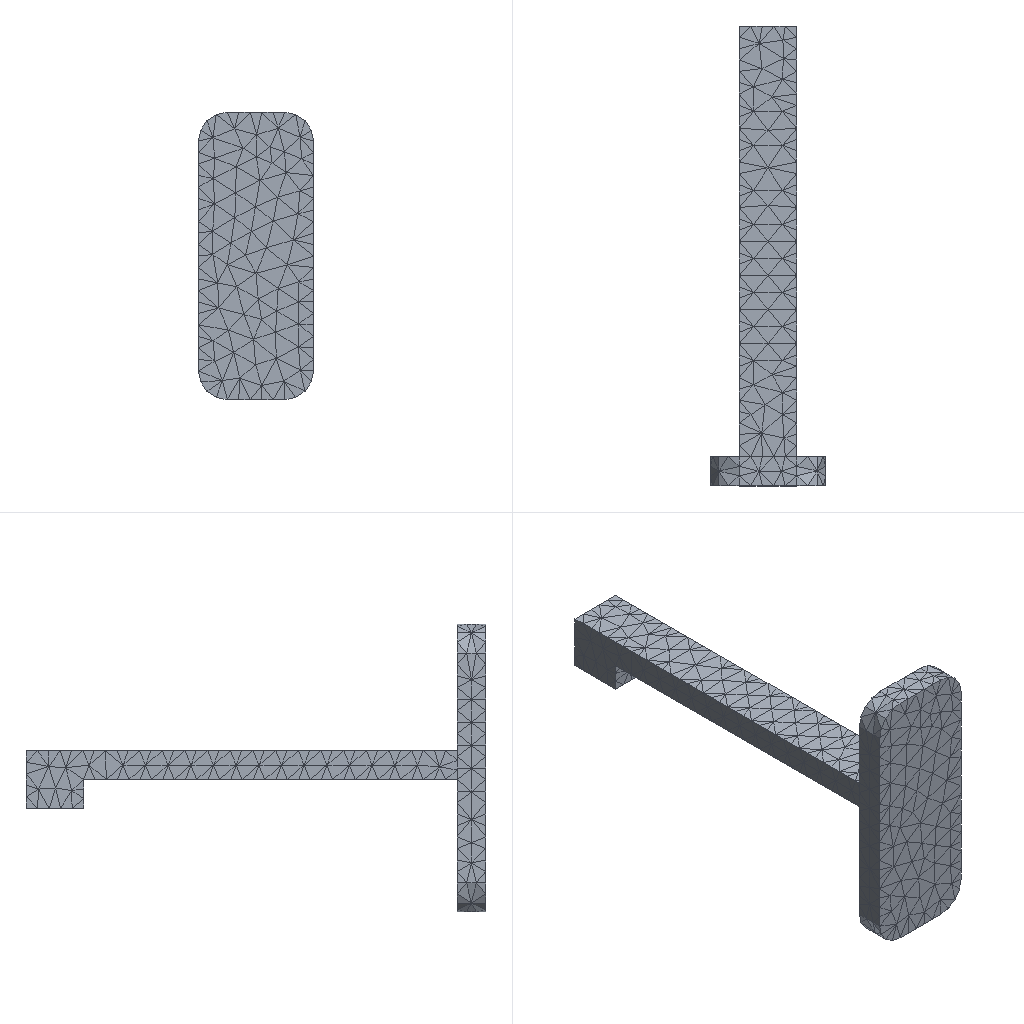Simulation study | ansys workbench
Ansys APDL input file, long lists of numbers shortened:
/batch
/config,noeldb,1     ! force off writing results to database
*get,_wallstrt,active,,time,wall
! ANSYS input file written by Workbench version 2021 R1
! File used for geometry attach:
/title,111111--____ (A5)
! ****** Begin Custom Load Command Snippet ******
/COM, ACT Extensions:
/COM,     LSDYNA, 2021.1
/COM,
! ****** End   Custom Load Command Snippet ******
*DIM,_wb_ProjectScratch_dir,string,248
_wb_ProjectScratch_dir(1) = ''
*DIM,_wb_SolverFiles_dir,string,248
_wb_SolverFiles_dir(1) = ''
*DIM,_wb_userfiles_dir,string,248
_wb_userfiles_dir(1) = ''
/com,--- Data in consistent NMM units. See Solving Units in the help system for more information.
/units,MPA
/nopr
/wb,file,start              !  signify a WB generated input file
/prep7
! Turn off shape checking because checks already performed inside WB mesher.
! See help system for more information.
SHPP,OFF,,NOWARN
/nolist
etcon,set             ! allow ANSYS to choose best KEYOP's for 180x elements, resets any applicable keyopt to MAPDL defaults
/com,*********** Nodes for the whole assembly ***********
nblock,3,,4436
(1i9,3e20.9e3)
        1     5.000000000E+00     8.000000000E+01    -3.200000000E+01
! (4032 more lines like these left out)
-1
/wb,elem,start            !  set before creation of elements
/com,*********** Elements for Body 1 "SYS-2\__" ***********
et,1,187
eblock,19,solid,,1982
(19i9)
        1        1        1        1        0        0        0        0       10        0        1      543      588      719      661     3482     3718     3487     3483
! (3963 more lines like these left out)
-1
/wb,elem,end               !  done creating elements
/com,*********** Send User Defined Coordinate System(s) ***********
csys,0
toffst,273.15,  ! Temperature offset from absolute zero
/com,*********** Set Reference Temperature ***********
tref,22.
/wb,mat,start              !  starting to send materials
/com,*********** Send Materials ***********
Temperature = 'TEMP' ! Temperature
MP,DENS,1,7.85e-09,	! tonne mm^-3
MP,ALPX,1,1.2e-05,	! C^-1
MP,C,1,434000000,	! mm^2 s^-2 C^-1
MP,KXX,1,60.5,	! tonne mm s^-3 C^-1
MP,RSVX,1,0.00017,	! ohm mm
MP,EX,1,200000,	! tonne s^-2 mm^-1
MP,NUXY,1,0.3,
MP,MURX,1,10000,
/wb,mat,end                !  done sending materials
!************************* Model Summary ********************
!SYS-2\__,	304,	matid,	1
!************************* End Model Summary ********************
! get the diagonal of the bounding box. Needed later for other things
*get,_xmin,node,,mnloc,x
*get,_ymin,node,,mnloc,y
*get,_zmin,node,,mnloc,z
*get,_xmax,node,,mxloc,x
*get,_ymax,node,,mxloc,y
*get,_zmax,node,,mxloc,z
_ASMDIAG=(_xmax-_xmin)*(_xmax-_xmin)+(_ymax-_ymin)*(_ymax-_ymin)+(_zmax-_zmin)*(_zmax-_zmin)
_ASMDIAG=SQRT(_ASMDIAG)
/wb,contact,start          !  starting to send contact
/wb,contact,end            !  done creating contacts
/golist
/wb,load,start             !  starting to send loads
/com,*********** Fixed Supports ***********
CMBLOCK,_FIXEDSU,NODE,      431
(8i10)
       265       268       269       270       271       272       275       278
! (53 more lines like these left out)
cmsel,s,_FIXEDSU
d,all,all
nsel,all
/com,*********** Define Force Using Surface Effect Elements ***********
local,12,0,0.,0.,0.,0.,0.,0.
csys,0
et,2,154
eblock,10,,,28
(15i9)
     3211        2        2        2       12        9      578      579      579      760     3650      579      761
! (27 more lines like these left out)
-1
esel,s,type,,2
keyop,2,2,1                ! Apply load in local coordinate system
keyop,2,7,1                ! Use original area so load is constant in large deformation
esel,all
/gst,on,on
fini
*get,_numnode,node,0,count
*get,_numelem,elem,0,count
*get, _MAXELEMNUM, elem, 0, NUM, MAX
*get, _MAXNODENUM, node, 0, NUM, MAX
*get, _MAXELEMTYPE, etyp, 0, NUM, MAX
*get, _MAXREALCONST, real, 0, NUM, MAX
/go
/wb,load,end               !  done creating loads
/com,--- Number of total nodes = %_numnode%
/com,--- Number of contact elements = 28
/com,--- Number of spring elements = 0
/com,--- Number of bearing elements = 0
/com,--- Number of solid elements = 1982
/com,--- Number of condensed parts = 0
/com,--- Number of total elements = %_numelem%
*get,_wallbsol,active,,time,wall
/com,****************************************************************************
/com,*************************    SOLUTION       ********************************
/com,****************************************************************************
/solu
antype,0                   ! static analysis
_thickRatio=  0     ! Ratio of thick parts in the model
eqsl,sparse,,,,,1
cntr,print,1               ! print out contact info and also make no initial contact an error
dmpoption,emat,no             ! Don't combine emat file for DANSYS
dmpoption,esav,no             ! Don't combine esav file for DANSYS
nldiag,cont,iter           ! print out contact info each equilibrium iteration
rescontrol,,none                 ! Do not keep any restart files
/com,****************************************************
/com,******************* SOLVE FOR LS 1 OF 1 ****************
esel,s,type,,2
nsle
sfe,all,1,pres,1,0.
sfe,all,2,pres,1,0.
sfe,all,3,pres,1,5.
nsel,all
esel,all
/nopr
/gopr
/nolist
nsub,1,1,1
time,1.
outres,erase
outres,all,none
outres,nsol,all,
outres,rsol,all
outres,eangl,all
outres,etmp,all
outres,veng,all
outres,strs,all,
outres,epel,all,
outres,eppl,all,
outres,cont,all,
! *********** WB SOLVE COMMAND ***********
! check interactive state
*get,ANSINTER_,active,,int
*if,ANSINTER_,ne,0,then
/eof
*endif
solve
/com *************** Write FE CONNECTORS *********
CEWRITE,file,ce,,INTE
/com,****************************************************
/com,*************** FINISHED SOLVE FOR LS 1 *************
*get,_wallasol,active,,time,wall
/nopr
*get,_numnode,node,0,count
*get,_numelem,elem,0,count
*get, _MAXELEMNUM, elem, 0, NUM, MAX
*get, _MAXNODENUM, node, 0, NUM, MAX,,,INTERNAL
*get, _MAXELEMTYPE, etyp, 0, NUM, MAX
*get, _MAXREALCONST, real, 0, NUM, MAX
/gopr
/post1
xmlo,ENCODING,ISO-8859-1
xmlo,parm
/xml,parm,xml
fini
/gopr
*get,_walldone,active,,time,wall
_preptime=(_wallbsol-_wallstrt)*3600
_solvtime=(_wallasol-_wallbsol)*3600
_posttime=(_walldone-_wallasol)*3600
_totaltim=(_walldone-_wallstrt)*3600
*get,_dlbratio,active,0,solu,dlbr
*get,_combtime,active,0,solu,comb
/com,--- Total number of nodes = %_numnode%
/com,--- Total number of elements = %_numelem%
/com,--- Element load balance ratio = %_dlbratio%
/com,--- Time to combine distributed files = %_combtime%
/wb,file,end               ! done with WB generated input